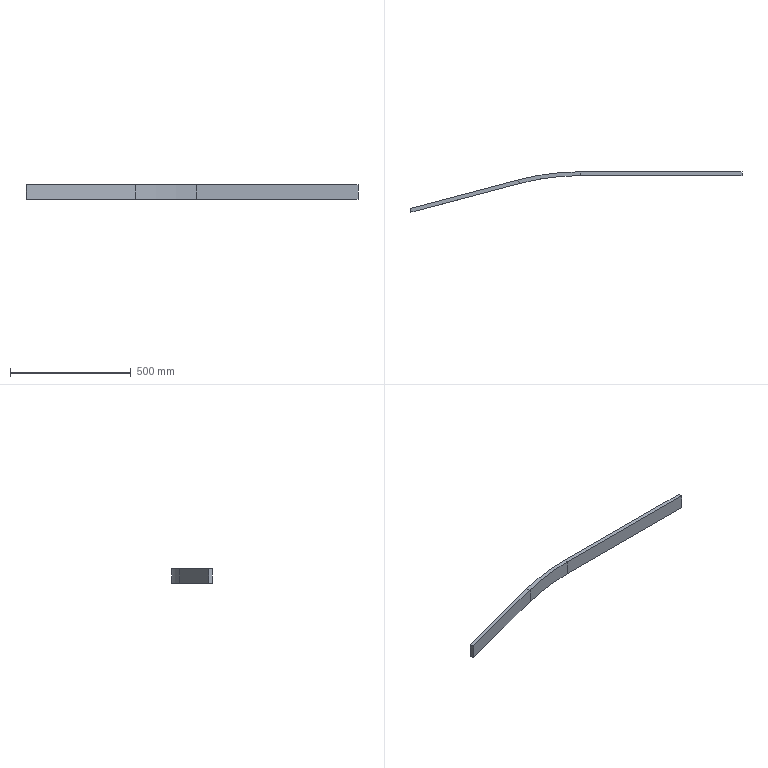Part | SolidWorks | features Extrusion 1, FlatPattern 1, SheetMetal 1, SolidToSheetMetal 1 | 1 solid | 14 faces | box 1376 x 167.7 x 60 mm | volume 1336375 mm3 | plane 12 | cylinder 2 | commonest cylinder face diameters 1968 x1 2000 x1
STEP:
#1=CARTESIAN_POINT('',(0.,0.,0.));
#2=VERTEX_POINT('',#1);
#3=CARTESIAN_POINT('',(0.,-16.,0.));
#4=VERTEX_POINT('',#3);
#5=CARTESIAN_POINT('',(0.,-16.,0.));
#6=DIRECTION('',(0.,-1.,0.));
#7=VECTOR('',#6,1000.);
#8=LINE('',#5,#7);
#9=EDGE_CURVE('',#2,#4,#8,.T.);
#10=ORIENTED_EDGE('',*,*,#9,.F.);
#11=CARTESIAN_POINT('',(0.,0.,60.));
#12=VERTEX_POINT('',#11);
#13=CARTESIAN_POINT('',(0.,0.,60.));
#14=DIRECTION('',(0.,0.,-1.));
#15=VECTOR('',#14,1000.);
#16=LINE('',#13,#15);
#17=EDGE_CURVE('',#12,#2,#16,.T.);
#18=ORIENTED_EDGE('',*,*,#17,.F.);
#19=CARTESIAN_POINT('',(0.,-16.,60.));
#20=VERTEX_POINT('',#19);
#21=CARTESIAN_POINT('',(0.,-16.,60.));
#22=DIRECTION('',(0.,-1.,0.));
#23=VECTOR('',#22,1000.);
#24=LINE('',#21,#23);
#25=EDGE_CURVE('',#12,#20,#24,.T.);
#26=ORIENTED_EDGE('',*,*,#25,.T.);
#27=CARTESIAN_POINT('',(0.,-16.,60.));
#28=DIRECTION('',(0.,0.,-1.));
#29=VECTOR('',#28,1000.);
#30=LINE('',#27,#29);
#31=EDGE_CURVE('',#20,#4,#30,.T.);
#32=ORIENTED_EDGE('',*,*,#31,.T.);
#33=EDGE_LOOP('',(#10,#18,#26,#32));
#34=FACE_OUTER_BOUND('',#33,.T.);
#35=CARTESIAN_POINT('',(0.,-16.,60.));
#36=DIRECTION('',(1.,0.,0.));
#37=DIRECTION('',(0.,0.,-1.));
#38=AXIS2_PLACEMENT_3D('',#35,#36,#37);
#39=PLANE('',#38);
#40=ADVANCED_FACE('',(#34),#39,.T.);
#41=ORIENTED_EDGE('',*,*,#25,.F.);
#42=CARTESIAN_POINT('',(-670.039,0.,60.));
#43=VERTEX_POINT('',#42);
#44=CARTESIAN_POINT('',(0.,0.,60.));
#45=DIRECTION('',(1.,0.,0.));
#46=VECTOR('',#45,1000.);
#47=LINE('',#44,#46);
#48=EDGE_CURVE('',#43,#12,#47,.T.);
#49=ORIENTED_EDGE('',*,*,#48,.F.);
#50=CARTESIAN_POINT('',(-670.039,-16.,60.));
#51=VERTEX_POINT('',#50);
#52=CARTESIAN_POINT('',(-670.039,-16.,60.));
#53=DIRECTION('',(0.,-1.,0.));
#54=VECTOR('',#53,1000.);
#55=LINE('',#52,#54);
#56=EDGE_CURVE('',#43,#51,#55,.T.);
#57=ORIENTED_EDGE('',*,*,#56,.T.);
#58=CARTESIAN_POINT('',(0.,-16.,60.));
#59=DIRECTION('',(1.,0.,0.));
#60=VECTOR('',#59,1000.);
#61=LINE('',#58,#60);
#62=EDGE_CURVE('',#51,#20,#61,.T.);
#63=ORIENTED_EDGE('',*,*,#62,.T.);
#64=EDGE_LOOP('',(#41,#49,#57,#63));
#65=FACE_OUTER_BOUND('',#64,.T.);
#66=CARTESIAN_POINT('',(0.,-16.,60.));
#67=DIRECTION('',(0.,0.,1.));
#68=DIRECTION('',(1.,0.,0.));
#69=AXIS2_PLACEMENT_3D('',#66,#67,#68);
#70=PLANE('',#69);
#71=ADVANCED_FACE('',(#65),#70,.T.);
#72=ORIENTED_EDGE('',*,*,#56,.F.);
#73=CARTESIAN_POINT('',(-925.644,-33.219,60.));
#74=VERTEX_POINT('',#73);
#75=CARTESIAN_POINT('',(-670.039,-1000.,60.));
#76=DIRECTION('',(0.,0.,-1.));
#77=DIRECTION('',(-1.,0.,0.));
#78=AXIS2_PLACEMENT_3D('',#75,#76,#77);
#79=CIRCLE('',#78,1000.);
#80=EDGE_CURVE('',#74,#43,#79,.T.);
#81=ORIENTED_EDGE('',*,*,#80,.F.);
#82=CARTESIAN_POINT('',(-921.554,-48.687,60.));
#83=VERTEX_POINT('',#82);
#84=CARTESIAN_POINT('',(-921.554,-48.687,60.));
#85=DIRECTION('',(0.2556,-0.9668,0.));
#86=VECTOR('',#85,1000.);
#87=LINE('',#84,#86);
#88=EDGE_CURVE('',#74,#83,#87,.T.);
#89=ORIENTED_EDGE('',*,*,#88,.T.);
#90=CARTESIAN_POINT('',(-670.039,-1000.,60.));
#91=DIRECTION('',(0.,0.,-1.));
#92=DIRECTION('',(-1.,0.,0.));
#93=AXIS2_PLACEMENT_3D('',#90,#91,#92);
#94=CIRCLE('',#93,984.);
#95=EDGE_CURVE('',#83,#51,#94,.T.);
#96=ORIENTED_EDGE('',*,*,#95,.T.);
#97=EDGE_LOOP('',(#72,#81,#89,#96));
#98=FACE_OUTER_BOUND('',#97,.T.);
#99=CARTESIAN_POINT('',(-670.039,-1000.,60.));
#100=DIRECTION('',(0.,0.,1.));
#101=DIRECTION('',(1.,0.,0.));
#102=AXIS2_PLACEMENT_3D('',#99,#100,#101);
#103=PLANE('',#102);
#104=ADVANCED_FACE('',(#98),#103,.T.);
#105=ORIENTED_EDGE('',*,*,#88,.F.);
#106=CARTESIAN_POINT('',(-1375.79,-152.231,60.));
#107=VERTEX_POINT('',#106);
#108=CARTESIAN_POINT('',(-925.644,-33.219,60.));
#109=DIRECTION('',(0.9668,0.2556,0.));
#110=VECTOR('',#109,1000.);
#111=LINE('',#108,#110);
#112=EDGE_CURVE('',#107,#74,#111,.T.);
#113=ORIENTED_EDGE('',*,*,#112,.F.);
#114=CARTESIAN_POINT('',(-1371.7,-167.7,60.));
#115=VERTEX_POINT('',#114);
#116=CARTESIAN_POINT('',(-1371.7,-167.7,60.));
#117=DIRECTION('',(0.2556,-0.9668,0.));
#118=VECTOR('',#117,1000.);
#119=LINE('',#116,#118);
#120=EDGE_CURVE('',#107,#115,#119,.T.);
#121=ORIENTED_EDGE('',*,*,#120,.T.);
#122=CARTESIAN_POINT('',(-921.554,-48.687,60.));
#123=DIRECTION('',(0.9668,0.2556,0.));
#124=VECTOR('',#123,1000.);
#125=LINE('',#122,#124);
#126=EDGE_CURVE('',#115,#83,#125,.T.);
#127=ORIENTED_EDGE('',*,*,#126,.T.);
#128=EDGE_LOOP('',(#105,#113,#121,#127));
#129=FACE_OUTER_BOUND('',#128,.T.);
#130=CARTESIAN_POINT('',(-921.554,-48.687,60.));
#131=DIRECTION('',(0.,0.,1.));
#132=DIRECTION('',(0.9668,0.2556,0.));
#133=AXIS2_PLACEMENT_3D('',#130,#131,#132);
#134=PLANE('',#133);
#135=ADVANCED_FACE('',(#129),#134,.T.);
#136=ORIENTED_EDGE('',*,*,#120,.F.);
#137=CARTESIAN_POINT('',(-1375.79,-152.231,0.));
#138=VERTEX_POINT('',#137);
#139=CARTESIAN_POINT('',(-1375.79,-152.231,60.));
#140=DIRECTION('',(0.,0.,-1.));
#141=VECTOR('',#140,1000.);
#142=LINE('',#139,#141);
#143=EDGE_CURVE('',#107,#138,#142,.T.);
#144=ORIENTED_EDGE('',*,*,#143,.T.);
#145=CARTESIAN_POINT('',(-1371.7,-167.7,0.));
#146=VERTEX_POINT('',#145);
#147=CARTESIAN_POINT('',(-1371.7,-167.7,0.));
#148=DIRECTION('',(0.2556,-0.9668,0.));
#149=VECTOR('',#148,1000.);
#150=LINE('',#147,#149);
#151=EDGE_CURVE('',#138,#146,#150,.T.);
#152=ORIENTED_EDGE('',*,*,#151,.T.);
#153=CARTESIAN_POINT('',(-1371.7,-167.7,60.));
#154=DIRECTION('',(0.,0.,-1.));
#155=VECTOR('',#154,1000.);
#156=LINE('',#153,#155);
#157=EDGE_CURVE('',#115,#146,#156,.T.);
#158=ORIENTED_EDGE('',*,*,#157,.F.);
#159=EDGE_LOOP('',(#136,#144,#152,#158));
#160=FACE_OUTER_BOUND('',#159,.T.);
#161=CARTESIAN_POINT('',(-1371.7,-167.7,60.));
#162=DIRECTION('',(0.9668,0.2556,0.));
#163=DIRECTION('',(0.,0.,-1.));
#164=AXIS2_PLACEMENT_3D('',#161,#162,#163);
#165=PLANE('',#164);
#166=ADVANCED_FACE('',(#160),#165,.F.);
#167=ORIENTED_EDGE('',*,*,#151,.F.);
#168=CARTESIAN_POINT('',(-925.644,-33.219,0.));
#169=VERTEX_POINT('',#168);
#170=CARTESIAN_POINT('',(-925.644,-33.219,0.));
#171=DIRECTION('',(0.9668,0.2556,0.));
#172=VECTOR('',#171,1000.);
#173=LINE('',#170,#172);
#174=EDGE_CURVE('',#138,#169,#173,.T.);
#175=ORIENTED_EDGE('',*,*,#174,.T.);
#176=CARTESIAN_POINT('',(-921.554,-48.687,0.));
#177=VERTEX_POINT('',#176);
#178=CARTESIAN_POINT('',(-921.554,-48.687,0.));
#179=DIRECTION('',(0.2556,-0.9668,0.));
#180=VECTOR('',#179,1000.);
#181=LINE('',#178,#180);
#182=EDGE_CURVE('',#169,#177,#181,.T.);
#183=ORIENTED_EDGE('',*,*,#182,.T.);
#184=CARTESIAN_POINT('',(-921.554,-48.687,0.));
#185=DIRECTION('',(0.9668,0.2556,0.));
#186=VECTOR('',#185,1000.);
#187=LINE('',#184,#186);
#188=EDGE_CURVE('',#146,#177,#187,.T.);
#189=ORIENTED_EDGE('',*,*,#188,.F.);
#190=EDGE_LOOP('',(#167,#175,#183,#189));
#191=FACE_OUTER_BOUND('',#190,.T.);
#192=CARTESIAN_POINT('',(-921.554,-48.687,0.));
#193=DIRECTION('',(0.,0.,1.));
#194=DIRECTION('',(0.9668,0.2556,0.));
#195=AXIS2_PLACEMENT_3D('',#192,#193,#194);
#196=PLANE('',#195);
#197=ADVANCED_FACE('',(#191),#196,.F.);
#198=ORIENTED_EDGE('',*,*,#182,.F.);
#199=CARTESIAN_POINT('',(-670.039,0.,0.));
#200=VERTEX_POINT('',#199);
#201=CARTESIAN_POINT('',(-670.039,-1000.,0.));
#202=DIRECTION('',(0.,0.,-1.));
#203=DIRECTION('',(-1.,0.,0.));
#204=AXIS2_PLACEMENT_3D('',#201,#202,#203);
#205=CIRCLE('',#204,1000.);
#206=EDGE_CURVE('',#169,#200,#205,.T.);
#207=ORIENTED_EDGE('',*,*,#206,.T.);
#208=CARTESIAN_POINT('',(-670.039,-16.,0.));
#209=VERTEX_POINT('',#208);
#210=CARTESIAN_POINT('',(-670.039,-16.,0.));
#211=DIRECTION('',(0.,-1.,0.));
#212=VECTOR('',#211,1000.);
#213=LINE('',#210,#212);
#214=EDGE_CURVE('',#200,#209,#213,.T.);
#215=ORIENTED_EDGE('',*,*,#214,.T.);
#216=CARTESIAN_POINT('',(-670.039,-1000.,0.));
#217=DIRECTION('',(0.,0.,-1.));
#218=DIRECTION('',(-1.,0.,0.));
#219=AXIS2_PLACEMENT_3D('',#216,#217,#218);
#220=CIRCLE('',#219,984.);
#221=EDGE_CURVE('',#177,#209,#220,.T.);
#222=ORIENTED_EDGE('',*,*,#221,.F.);
#223=EDGE_LOOP('',(#198,#207,#215,#222));
#224=FACE_OUTER_BOUND('',#223,.T.);
#225=CARTESIAN_POINT('',(-670.039,-1000.,0.));
#226=DIRECTION('',(0.,0.,1.));
#227=DIRECTION('',(1.,0.,0.));
#228=AXIS2_PLACEMENT_3D('',#225,#226,#227);
#229=PLANE('',#228);
#230=ADVANCED_FACE('',(#224),#229,.F.);
#231=ORIENTED_EDGE('',*,*,#221,.T.);
#232=CARTESIAN_POINT('',(-670.039,-16.,60.));
#233=DIRECTION('',(0.,0.,-1.));
#234=VECTOR('',#233,1000.);
#235=LINE('',#232,#234);
#236=EDGE_CURVE('',#51,#209,#235,.T.);
#237=ORIENTED_EDGE('',*,*,#236,.F.);
#238=ORIENTED_EDGE('',*,*,#95,.F.);
#239=CARTESIAN_POINT('',(-921.554,-48.687,60.));
#240=DIRECTION('',(0.,0.,-1.));
#241=VECTOR('',#240,1000.);
#242=LINE('',#239,#241);
#243=EDGE_CURVE('',#83,#177,#242,.T.);
#244=ORIENTED_EDGE('',*,*,#243,.T.);
#245=EDGE_LOOP('',(#231,#237,#238,#244));
#246=FACE_OUTER_BOUND('',#245,.T.);
#247=CARTESIAN_POINT('',(-670.039,-1000.,60.));
#248=DIRECTION('',(0.,0.,-1.));
#249=DIRECTION('',(-1.,0.,0.));
#250=AXIS2_PLACEMENT_3D('',#247,#248,#249);
#251=CYLINDRICAL_SURFACE('',#250,984.);
#252=ADVANCED_FACE('',(#246),#251,.F.);
#253=ORIENTED_EDGE('',*,*,#188,.T.);
#254=ORIENTED_EDGE('',*,*,#243,.F.);
#255=ORIENTED_EDGE('',*,*,#126,.F.);
#256=ORIENTED_EDGE('',*,*,#157,.T.);
#257=EDGE_LOOP('',(#253,#254,#255,#256));
#258=FACE_OUTER_BOUND('',#257,.T.);
#259=CARTESIAN_POINT('',(-921.554,-48.687,60.));
#260=DIRECTION('',(-0.2556,0.9668,0.));
#261=DIRECTION('',(-0.9668,-0.2556,0.));
#262=AXIS2_PLACEMENT_3D('',#259,#260,#261);
#263=PLANE('',#262);
#264=ADVANCED_FACE('',(#258),#263,.F.);
#265=CARTESIAN_POINT('',(0.,-16.,0.));
#266=DIRECTION('',(1.,0.,0.));
#267=VECTOR('',#266,1000.);
#268=LINE('',#265,#267);
#269=EDGE_CURVE('',#209,#4,#268,.T.);
#270=ORIENTED_EDGE('',*,*,#269,.T.);
#271=ORIENTED_EDGE('',*,*,#31,.F.);
#272=ORIENTED_EDGE('',*,*,#62,.F.);
#273=ORIENTED_EDGE('',*,*,#236,.T.);
#274=EDGE_LOOP('',(#270,#271,#272,#273));
#275=FACE_OUTER_BOUND('',#274,.T.);
#276=CARTESIAN_POINT('',(0.,-16.,60.));
#277=DIRECTION('',(0.,1.,0.));
#278=DIRECTION('',(-1.,0.,0.));
#279=AXIS2_PLACEMENT_3D('',#276,#277,#278);
#280=PLANE('',#279);
#281=ADVANCED_FACE('',(#275),#280,.F.);
#282=CARTESIAN_POINT('',(0.,0.,0.));
#283=DIRECTION('',(1.,0.,0.));
#284=VECTOR('',#283,1000.);
#285=LINE('',#282,#284);
#286=EDGE_CURVE('',#200,#2,#285,.T.);
#287=ORIENTED_EDGE('',*,*,#286,.T.);
#288=ORIENTED_EDGE('',*,*,#9,.T.);
#289=ORIENTED_EDGE('',*,*,#269,.F.);
#290=ORIENTED_EDGE('',*,*,#214,.F.);
#291=EDGE_LOOP('',(#287,#288,#289,#290));
#292=FACE_OUTER_BOUND('',#291,.T.);
#293=CARTESIAN_POINT('',(0.,-16.,0.));
#294=DIRECTION('',(0.,0.,1.));
#295=DIRECTION('',(1.,0.,0.));
#296=AXIS2_PLACEMENT_3D('',#293,#294,#295);
#297=PLANE('',#296);
#298=ADVANCED_FACE('',(#292),#297,.F.);
#299=ORIENTED_EDGE('',*,*,#206,.F.);
#300=CARTESIAN_POINT('',(-925.644,-33.219,60.));
#301=DIRECTION('',(0.,0.,-1.));
#302=VECTOR('',#301,1000.);
#303=LINE('',#300,#302);
#304=EDGE_CURVE('',#74,#169,#303,.T.);
#305=ORIENTED_EDGE('',*,*,#304,.F.);
#306=ORIENTED_EDGE('',*,*,#80,.T.);
#307=CARTESIAN_POINT('',(-670.039,0.,60.));
#308=DIRECTION('',(0.,0.,-1.));
#309=VECTOR('',#308,1000.);
#310=LINE('',#307,#309);
#311=EDGE_CURVE('',#43,#200,#310,.T.);
#312=ORIENTED_EDGE('',*,*,#311,.T.);
#313=EDGE_LOOP('',(#299,#305,#306,#312));
#314=FACE_OUTER_BOUND('',#313,.T.);
#315=CARTESIAN_POINT('',(-670.039,-1000.,60.));
#316=DIRECTION('',(0.,0.,-1.));
#317=DIRECTION('',(-1.,0.,0.));
#318=AXIS2_PLACEMENT_3D('',#315,#316,#317);
#319=CYLINDRICAL_SURFACE('',#318,1000.);
#320=ADVANCED_FACE('',(#314),#319,.T.);
#321=ORIENTED_EDGE('',*,*,#174,.F.);
#322=ORIENTED_EDGE('',*,*,#143,.F.);
#323=ORIENTED_EDGE('',*,*,#112,.T.);
#324=ORIENTED_EDGE('',*,*,#304,.T.);
#325=EDGE_LOOP('',(#321,#322,#323,#324));
#326=FACE_OUTER_BOUND('',#325,.T.);
#327=CARTESIAN_POINT('',(-925.644,-33.219,60.));
#328=DIRECTION('',(-0.2556,0.9668,0.));
#329=DIRECTION('',(-0.9668,-0.2556,0.));
#330=AXIS2_PLACEMENT_3D('',#327,#328,#329);
#331=PLANE('',#330);
#332=ADVANCED_FACE('',(#326),#331,.T.);
#333=ORIENTED_EDGE('',*,*,#286,.F.);
#334=ORIENTED_EDGE('',*,*,#311,.F.);
#335=ORIENTED_EDGE('',*,*,#48,.T.);
#336=ORIENTED_EDGE('',*,*,#17,.T.);
#337=EDGE_LOOP('',(#333,#334,#335,#336));
#338=FACE_OUTER_BOUND('',#337,.T.);
#339=CARTESIAN_POINT('',(0.,0.,60.));
#340=DIRECTION('',(0.,1.,0.));
#341=DIRECTION('',(-1.,0.,0.));
#342=AXIS2_PLACEMENT_3D('',#339,#340,#341);
#343=PLANE('',#342);
#344=ADVANCED_FACE('',(#338),#343,.T.);
#345=CLOSED_SHELL('',(#40,#71,#104,#135,#166,#197,#230,#252,#264,#281,#298,#320,#332,#344));
#346=MANIFOLD_SOLID_BREP('',#345);
#347=CARTESIAN_POINT('',(0.,0.,0.));
#348=DIRECTION('',(0.,0.,1.));
#349=DIRECTION('',(1.,0.,0.));
#350=AXIS2_PLACEMENT_3D('',#347,#348,#349);
#351=(LENGTH_UNIT()NAMED_UNIT(*)SI_UNIT(.MILLI.,.METRE.));
#352=UNCERTAINTY_MEASURE_WITH_UNIT(LENGTH_MEASURE(0.00001),#351,'','');
#353=(NAMED_UNIT(*)PLANE_ANGLE_UNIT()SI_UNIT($,.RADIAN.));
#354=(NAMED_UNIT(*)SI_UNIT($,.STERADIAN.)SOLID_ANGLE_UNIT());
#355=(GEOMETRIC_REPRESENTATION_CONTEXT(3)GLOBAL_UNCERTAINTY_ASSIGNED_CONTEXT((#352))GLOBAL_UNIT_ASSIGNED_CONTEXT((#351,#353,#354))REPRESENTATION_CONTEXT('',''));
#356=ADVANCED_BREP_SHAPE_REPRESENTATION('',(#346,#350),#355);